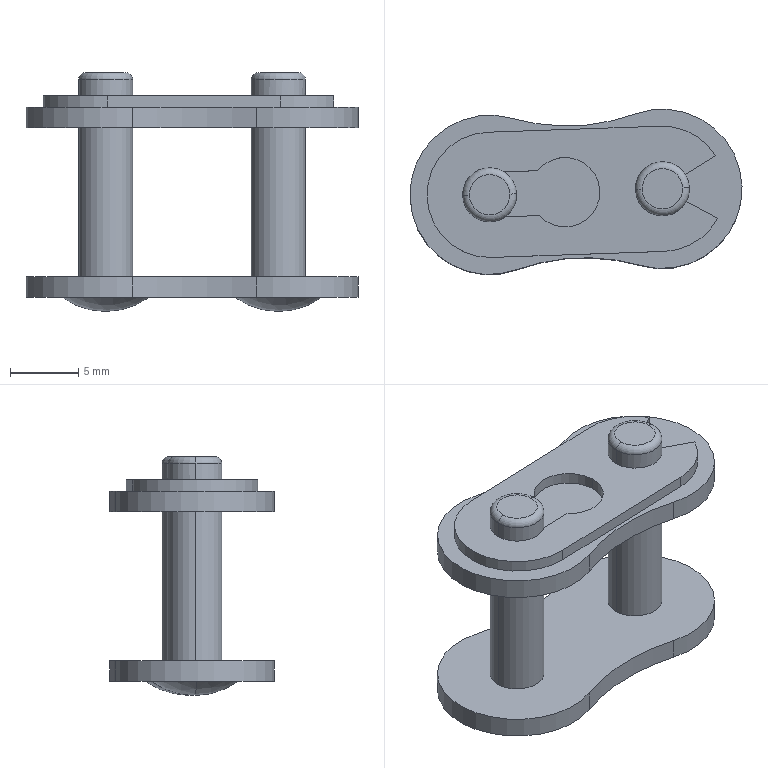Part | STEP file | CHES40-46-Part-12 | 1 solid | 45 faces | box 24.392 x 12.143 x 17.55 mm | volume 1198 mm3 | cylinder 23 | plane 14 | torus 4 | sphere 4 | commonest cylinder face diameters 3.97 x8 11.7 x6 29.64 x4 9.2 x3 5.1 x2
STEP:
#1=CARTESIAN_POINT('',(-191.992,69.511,9.53));
#2=VERTEX_POINT('',#1);
#3=CARTESIAN_POINT('',(-189.024,69.615,9.53));
#4=VERTEX_POINT('',#3);
#5=CARTESIAN_POINT('',(-190.508,69.563,9.53));
#6=DIRECTION('',(0.,0.,1.));
#7=DIRECTION('',(0.9994,0.0349,0.));
#8=AXIS2_PLACEMENT_3D('',#5,#6,#7);
#9=CIRCLE('',#8,1.485);
#10=EDGE_CURVE('',#2,#4,#9,.T.);
#11=ORIENTED_EDGE('',*,*,#10,.F.);
#12=CARTESIAN_POINT('',(-192.492,69.494,9.03));
#13=VERTEX_POINT('',#12);
#14=CARTESIAN_POINT('',(-191.992,69.511,9.03));
#15=DIRECTION('',(0.0349,-0.9994,0.));
#16=DIRECTION('',(0.9994,0.0349,0.));
#17=AXIS2_PLACEMENT_3D('',#14,#15,#16);
#18=CIRCLE('',#17,0.5);
#19=EDGE_CURVE('',#2,#13,#18,.T.);
#20=ORIENTED_EDGE('',*,*,#19,.T.);
#21=CARTESIAN_POINT('',(-188.524,69.632,9.03));
#22=VERTEX_POINT('',#21);
#23=CARTESIAN_POINT('',(-190.508,69.563,9.03));
#24=DIRECTION('',(0.,0.,-1.));
#25=DIRECTION('',(0.9994,0.0349,0.));
#26=AXIS2_PLACEMENT_3D('',#23,#24,#25);
#27=CIRCLE('',#26,1.985);
#28=EDGE_CURVE('',#22,#13,#27,.T.);
#29=ORIENTED_EDGE('',*,*,#28,.F.);
#30=CARTESIAN_POINT('',(-189.024,69.615,9.03));
#31=DIRECTION('',(-0.0349,0.9994,0.));
#32=DIRECTION('',(-0.9994,-0.0349,0.));
#33=AXIS2_PLACEMENT_3D('',#30,#31,#32);
#34=CIRCLE('',#33,0.5);
#35=EDGE_CURVE('',#4,#22,#34,.T.);
#36=ORIENTED_EDGE('',*,*,#35,.F.);
#37=EDGE_LOOP('',(#11,#20,#29,#36));
#38=FACE_OUTER_BOUND('',#37,.T.);
#39=CARTESIAN_POINT('',(-190.508,69.563,9.03));
#40=DIRECTION('',(0.,0.,-1.));
#41=DIRECTION('',(0.9994,0.0349,0.));
#42=AXIS2_PLACEMENT_3D('',#39,#40,#41);
#43=TOROIDAL_SURFACE('',#42,1.485,0.5);
#44=ADVANCED_FACE('',(#38),#43,.T.);
#45=CARTESIAN_POINT('',(-204.684,69.068,9.53));
#46=VERTEX_POINT('',#45);
#47=CARTESIAN_POINT('',(-201.716,69.172,9.53));
#48=VERTEX_POINT('',#47);
#49=CARTESIAN_POINT('',(-203.2,69.12,9.53));
#50=DIRECTION('',(0.,0.,1.));
#51=DIRECTION('',(0.9994,0.0349,0.));
#52=AXIS2_PLACEMENT_3D('',#49,#50,#51);
#53=CIRCLE('',#52,1.485);
#54=EDGE_CURVE('',#46,#48,#53,.T.);
#55=ORIENTED_EDGE('',*,*,#54,.F.);
#56=CARTESIAN_POINT('',(-205.184,69.051,9.03));
#57=VERTEX_POINT('',#56);
#58=CARTESIAN_POINT('',(-204.684,69.068,9.03));
#59=DIRECTION('',(0.0349,-0.9994,0.));
#60=DIRECTION('',(0.9994,0.0349,0.));
#61=AXIS2_PLACEMENT_3D('',#58,#59,#60);
#62=CIRCLE('',#61,0.5);
#63=EDGE_CURVE('',#46,#57,#62,.T.);
#64=ORIENTED_EDGE('',*,*,#63,.T.);
#65=CARTESIAN_POINT('',(-201.216,69.189,9.03));
#66=VERTEX_POINT('',#65);
#67=CARTESIAN_POINT('',(-203.2,69.12,9.03));
#68=DIRECTION('',(0.,0.,-1.));
#69=DIRECTION('',(0.9994,0.0349,0.));
#70=AXIS2_PLACEMENT_3D('',#67,#68,#69);
#71=CIRCLE('',#70,1.985);
#72=EDGE_CURVE('',#66,#57,#71,.T.);
#73=ORIENTED_EDGE('',*,*,#72,.F.);
#74=CARTESIAN_POINT('',(-201.716,69.172,9.03));
#75=DIRECTION('',(-0.0349,0.9994,0.));
#76=DIRECTION('',(-0.9994,-0.0349,0.));
#77=AXIS2_PLACEMENT_3D('',#74,#75,#76);
#78=CIRCLE('',#77,0.5);
#79=EDGE_CURVE('',#48,#66,#78,.T.);
#80=ORIENTED_EDGE('',*,*,#79,.F.);
#81=EDGE_LOOP('',(#55,#64,#73,#80));
#82=FACE_OUTER_BOUND('',#81,.T.);
#83=CARTESIAN_POINT('',(-203.2,69.12,9.03));
#84=DIRECTION('',(0.,0.,-1.));
#85=DIRECTION('',(0.9994,0.0349,0.));
#86=AXIS2_PLACEMENT_3D('',#83,#84,#85);
#87=TOROIDAL_SURFACE('',#86,1.485,0.5);
#88=ADVANCED_FACE('',(#82),#87,.T.);
#89=ORIENTED_EDGE('',*,*,#72,.T.);
#90=CARTESIAN_POINT('',(-205.184,69.051,7.825));
#91=VERTEX_POINT('',#90);
#92=CARTESIAN_POINT('',(-205.184,69.051,-8.02));
#93=DIRECTION('',(0.,0.,-1.));
#94=VECTOR('',#93,1000.);
#95=LINE('',#92,#94);
#96=EDGE_CURVE('',#57,#91,#95,.T.);
#97=ORIENTED_EDGE('',*,*,#96,.T.);
#98=CARTESIAN_POINT('',(-202.04,67.51,7.825));
#99=VERTEX_POINT('',#98);
#100=CARTESIAN_POINT('',(-203.2,69.12,7.825));
#101=DIRECTION('',(0.,0.,1.));
#102=DIRECTION('',(-0.9994,-0.0349,0.));
#103=AXIS2_PLACEMENT_3D('',#100,#101,#102);
#104=CIRCLE('',#103,1.985);
#105=EDGE_CURVE('',#91,#99,#104,.T.);
#106=ORIENTED_EDGE('',*,*,#105,.T.);
#107=CARTESIAN_POINT('',(-202.04,67.51,6.975));
#108=VERTEX_POINT('',#107);
#109=CARTESIAN_POINT('',(-202.04,67.51,7.825));
#110=DIRECTION('',(0.,0.,-1.));
#111=VECTOR('',#110,1000.);
#112=LINE('',#109,#111);
#113=EDGE_CURVE('',#99,#108,#112,.T.);
#114=ORIENTED_EDGE('',*,*,#113,.T.);
#115=CARTESIAN_POINT('',(-201.216,69.189,6.975));
#116=VERTEX_POINT('',#115);
#117=CARTESIAN_POINT('',(-203.2,69.12,6.975));
#118=DIRECTION('',(0.,0.,1.));
#119=DIRECTION('',(0.9994,0.0349,0.));
#120=AXIS2_PLACEMENT_3D('',#117,#118,#119);
#121=CIRCLE('',#120,1.985);
#122=EDGE_CURVE('',#108,#116,#121,.T.);
#123=ORIENTED_EDGE('',*,*,#122,.T.);
#124=CARTESIAN_POINT('',(-201.216,69.189,-8.02));
#125=DIRECTION('',(0.,0.,-1.));
#126=VECTOR('',#125,1000.);
#127=LINE('',#124,#126);
#128=EDGE_CURVE('',#66,#116,#127,.T.);
#129=ORIENTED_EDGE('',*,*,#128,.F.);
#130=EDGE_LOOP('',(#89,#97,#106,#114,#123,#129));
#131=FACE_OUTER_BOUND('',#130,.T.);
#132=CARTESIAN_POINT('',(-203.2,69.12,-8.02));
#133=DIRECTION('',(0.,0.,-1.));
#134=DIRECTION('',(0.9994,0.0349,0.));
#135=AXIS2_PLACEMENT_3D('',#132,#133,#134);
#136=CYLINDRICAL_SURFACE('',#135,1.985);
#137=ADVANCED_FACE('',(#131),#136,.T.);
#138=CARTESIAN_POINT('',(-199.539,67.597,7.825));
#139=VERTEX_POINT('',#138);
#140=CARTESIAN_POINT('',(-195.105,69.403,7.825));
#141=VERTEX_POINT('',#140);
#142=CARTESIAN_POINT('',(-197.653,69.314,7.825));
#143=DIRECTION('',(0.,0.,1.));
#144=DIRECTION('',(-0.9994,-0.0349,0.));
#145=AXIS2_PLACEMENT_3D('',#142,#143,#144);
#146=CIRCLE('',#145,2.55);
#147=EDGE_CURVE('',#139,#141,#146,.T.);
#148=ORIENTED_EDGE('',*,*,#147,.T.);
#149=CARTESIAN_POINT('',(-195.105,69.403,6.975));
#150=VERTEX_POINT('',#149);
#151=CARTESIAN_POINT('',(-195.105,69.403,7.825));
#152=DIRECTION('',(0.,0.,-1.));
#153=VECTOR('',#152,1000.);
#154=LINE('',#151,#153);
#155=EDGE_CURVE('',#141,#150,#154,.T.);
#156=ORIENTED_EDGE('',*,*,#155,.T.);
#157=CARTESIAN_POINT('',(-199.539,67.597,6.975));
#158=VERTEX_POINT('',#157);
#159=CARTESIAN_POINT('',(-197.653,69.314,6.975));
#160=DIRECTION('',(0.,0.,1.));
#161=DIRECTION('',(-0.9994,-0.0349,0.));
#162=AXIS2_PLACEMENT_3D('',#159,#160,#161);
#163=CIRCLE('',#162,2.55);
#164=EDGE_CURVE('',#158,#150,#163,.T.);
#165=ORIENTED_EDGE('',*,*,#164,.F.);
#166=CARTESIAN_POINT('',(-199.539,67.597,7.825));
#167=DIRECTION('',(0.,0.,-1.));
#168=VECTOR('',#167,1000.);
#169=LINE('',#166,#168);
#170=EDGE_CURVE('',#139,#158,#169,.T.);
#171=ORIENTED_EDGE('',*,*,#170,.F.);
#172=EDGE_LOOP('',(#148,#156,#165,#171));
#173=FACE_OUTER_BOUND('',#172,.T.);
#174=CARTESIAN_POINT('',(-197.653,69.314,7.825));
#175=DIRECTION('',(0.,0.,-1.));
#176=DIRECTION('',(0.9994,0.0349,0.));
#177=AXIS2_PLACEMENT_3D('',#174,#175,#176);
#178=CYLINDRICAL_SURFACE('',#177,2.55);
#179=ADVANCED_FACE('',(#173),#178,.F.);
#180=CARTESIAN_POINT('',(-187.31,69.675,-6.975));
#181=VERTEX_POINT('',#180);
#182=CARTESIAN_POINT('',(-193.706,69.452,-6.975));
#183=VERTEX_POINT('',#182);
#184=CARTESIAN_POINT('',(-190.508,69.563,-6.975));
#185=DIRECTION('',(0.,0.,1.));
#186=DIRECTION('',(-0.9994,-0.0349,0.));
#187=AXIS2_PLACEMENT_3D('',#184,#185,#186);
#188=CIRCLE('',#187,3.2);
#189=EDGE_CURVE('',#181,#183,#188,.T.);
#190=ORIENTED_EDGE('',*,*,#189,.F.);
#191=CARTESIAN_POINT('',(-190.508,69.563,-8.02));
#192=VERTEX_POINT('',#191);
#193=CARTESIAN_POINT('',(-190.508,69.563,-2.598));
#194=DIRECTION('',(-0.0349,0.9994,0.));
#195=DIRECTION('',(-0.9994,-0.0349,0.));
#196=AXIS2_PLACEMENT_3D('',#193,#194,#195);
#197=CIRCLE('',#196,5.422);
#198=EDGE_CURVE('',#181,#192,#197,.T.);
#199=ORIENTED_EDGE('',*,*,#198,.T.);
#200=CARTESIAN_POINT('',(-190.508,69.563,-2.598));
#201=DIRECTION('',(0.0349,-0.9994,0.));
#202=DIRECTION('',(0.9994,0.0349,0.));
#203=AXIS2_PLACEMENT_3D('',#200,#201,#202);
#204=CIRCLE('',#203,5.422);
#205=EDGE_CURVE('',#183,#192,#204,.T.);
#206=ORIENTED_EDGE('',*,*,#205,.F.);
#207=EDGE_LOOP('',(#190,#199,#206));
#208=FACE_OUTER_BOUND('',#207,.T.);
#209=CARTESIAN_POINT('',(-190.508,69.563,-2.598));
#210=DIRECTION('',(-0.0349,0.9994,0.));
#211=DIRECTION('',(-0.9994,-0.0349,0.));
#212=AXIS2_PLACEMENT_3D('',#209,#210,#211);
#213=SPHERICAL_SURFACE('',#212,5.422);
#214=ADVANCED_FACE('',(#208),#213,.T.);
#215=CARTESIAN_POINT('',(-200.002,69.232,-6.975));
#216=VERTEX_POINT('',#215);
#217=CARTESIAN_POINT('',(-206.398,69.008,-6.975));
#218=VERTEX_POINT('',#217);
#219=CARTESIAN_POINT('',(-203.2,69.12,-6.975));
#220=DIRECTION('',(0.,0.,1.));
#221=DIRECTION('',(-0.9994,-0.0349,0.));
#222=AXIS2_PLACEMENT_3D('',#219,#220,#221);
#223=CIRCLE('',#222,3.2);
#224=EDGE_CURVE('',#216,#218,#223,.T.);
#225=ORIENTED_EDGE('',*,*,#224,.F.);
#226=CARTESIAN_POINT('',(-203.2,69.12,-8.02));
#227=VERTEX_POINT('',#226);
#228=CARTESIAN_POINT('',(-203.2,69.12,-2.598));
#229=DIRECTION('',(-0.0349,0.9994,0.));
#230=DIRECTION('',(-0.9994,-0.0349,0.));
#231=AXIS2_PLACEMENT_3D('',#228,#229,#230);
#232=CIRCLE('',#231,5.422);
#233=EDGE_CURVE('',#216,#227,#232,.T.);
#234=ORIENTED_EDGE('',*,*,#233,.T.);
#235=CARTESIAN_POINT('',(-203.2,69.12,-2.598));
#236=DIRECTION('',(0.0349,-0.9994,0.));
#237=DIRECTION('',(0.9994,0.0349,0.));
#238=AXIS2_PLACEMENT_3D('',#235,#236,#237);
#239=CIRCLE('',#238,5.422);
#240=EDGE_CURVE('',#218,#227,#239,.T.);
#241=ORIENTED_EDGE('',*,*,#240,.F.);
#242=EDGE_LOOP('',(#225,#234,#241));
#243=FACE_OUTER_BOUND('',#242,.T.);
#244=CARTESIAN_POINT('',(-203.2,69.12,-2.598));
#245=DIRECTION('',(-0.0349,0.9994,0.));
#246=DIRECTION('',(-0.9994,-0.0349,0.));
#247=AXIS2_PLACEMENT_3D('',#244,#245,#246);
#248=SPHERICAL_SURFACE('',#247,5.422);
#249=ADVANCED_FACE('',(#243),#248,.T.);
#250=CARTESIAN_POINT('',(-184.661,69.767,-5.475));
#251=VERTEX_POINT('',#250);
#252=CARTESIAN_POINT('',(-192.498,75.064,-5.475));
#253=VERTEX_POINT('',#252);
#254=CARTESIAN_POINT('',(-190.508,69.563,-5.475));
#255=DIRECTION('',(0.,0.,1.));
#256=DIRECTION('',(-0.9994,-0.0349,0.));
#257=AXIS2_PLACEMENT_3D('',#254,#255,#256);
#258=CIRCLE('',#257,5.85);
#259=EDGE_CURVE('',#251,#253,#258,.T.);
#260=ORIENTED_EDGE('',*,*,#259,.F.);
#261=CARTESIAN_POINT('',(-184.661,69.767,-6.975));
#262=VERTEX_POINT('',#261);
#263=CARTESIAN_POINT('',(-184.661,69.767,-5.475));
#264=DIRECTION('',(0.,0.,-1.));
#265=VECTOR('',#264,1000.);
#266=LINE('',#263,#265);
#267=EDGE_CURVE('',#251,#262,#266,.T.);
#268=ORIENTED_EDGE('',*,*,#267,.T.);
#269=CARTESIAN_POINT('',(-192.498,75.064,-6.975));
#270=VERTEX_POINT('',#269);
#271=CARTESIAN_POINT('',(-190.508,69.563,-6.975));
#272=DIRECTION('',(0.,0.,1.));
#273=DIRECTION('',(-0.9994,-0.0349,0.));
#274=AXIS2_PLACEMENT_3D('',#271,#272,#273);
#275=CIRCLE('',#274,5.85);
#276=EDGE_CURVE('',#262,#270,#275,.T.);
#277=ORIENTED_EDGE('',*,*,#276,.T.);
#278=CARTESIAN_POINT('',(-192.498,75.064,-5.475));
#279=DIRECTION('',(0.,0.,-1.));
#280=VECTOR('',#279,1000.);
#281=LINE('',#278,#280);
#282=EDGE_CURVE('',#253,#270,#281,.T.);
#283=ORIENTED_EDGE('',*,*,#282,.F.);
#284=EDGE_LOOP('',(#260,#268,#277,#283));
#285=FACE_OUTER_BOUND('',#284,.T.);
#286=CARTESIAN_POINT('',(-190.508,69.563,-5.475));
#287=DIRECTION('',(0.,0.,-1.));
#288=DIRECTION('',(0.9994,0.0349,0.));
#289=AXIS2_PLACEMENT_3D('',#286,#287,#288);
#290=CYLINDRICAL_SURFACE('',#289,5.85);
#291=ADVANCED_FACE('',(#285),#290,.T.);
#292=CARTESIAN_POINT('',(-201.216,69.189,5.475));
#293=VERTEX_POINT('',#292);
#294=CARTESIAN_POINT('',(-205.184,69.051,5.475));
#295=VERTEX_POINT('',#294);
#296=CARTESIAN_POINT('',(-203.2,69.12,5.475));
#297=DIRECTION('',(0.,0.,-1.));
#298=DIRECTION('',(0.9994,0.0349,0.));
#299=AXIS2_PLACEMENT_3D('',#296,#297,#298);
#300=CIRCLE('',#299,1.985);
#301=EDGE_CURVE('',#293,#295,#300,.T.);
#302=ORIENTED_EDGE('',*,*,#301,.T.);
#303=CARTESIAN_POINT('',(-205.184,69.051,-5.475));
#304=VERTEX_POINT('',#303);
#305=CARTESIAN_POINT('',(-205.184,69.051,-8.02));
#306=DIRECTION('',(0.,0.,-1.));
#307=VECTOR('',#306,1000.);
#308=LINE('',#305,#307);
#309=EDGE_CURVE('',#295,#304,#308,.T.);
#310=ORIENTED_EDGE('',*,*,#309,.T.);
#311=CARTESIAN_POINT('',(-201.216,69.189,-5.475));
#312=VERTEX_POINT('',#311);
#313=CARTESIAN_POINT('',(-203.2,69.12,-5.475));
#314=DIRECTION('',(0.,0.,1.));
#315=DIRECTION('',(-0.9994,-0.0349,0.));
#316=AXIS2_PLACEMENT_3D('',#313,#314,#315);
#317=CIRCLE('',#316,1.985);
#318=EDGE_CURVE('',#304,#312,#317,.T.);
#319=ORIENTED_EDGE('',*,*,#318,.T.);
#320=CARTESIAN_POINT('',(-201.216,69.189,-8.02));
#321=DIRECTION('',(0.,0.,-1.));
#322=VECTOR('',#321,1000.);
#323=LINE('',#320,#322);
#324=EDGE_CURVE('',#293,#312,#323,.T.);
#325=ORIENTED_EDGE('',*,*,#324,.F.);
#326=EDGE_LOOP('',(#302,#310,#319,#325));
#327=FACE_OUTER_BOUND('',#326,.T.);
#328=CARTESIAN_POINT('',(-203.2,69.12,-8.02));
#329=DIRECTION('',(0.,0.,-1.));
#330=DIRECTION('',(0.9994,0.0349,0.));
#331=AXIS2_PLACEMENT_3D('',#328,#329,#330);
#332=CYLINDRICAL_SURFACE('',#331,1.985);
#333=ADVANCED_FACE('',(#327),#332,.T.);
#334=ORIENTED_EDGE('',*,*,#28,.T.);
#335=CARTESIAN_POINT('',(-192.492,69.494,7.825));
#336=VERTEX_POINT('',#335);
#337=CARTESIAN_POINT('',(-192.492,69.494,-8.02));
#338=DIRECTION('',(0.,0.,-1.));
#339=VECTOR('',#338,1000.);
#340=LINE('',#337,#339);
#341=EDGE_CURVE('',#13,#336,#340,.T.);
#342=ORIENTED_EDGE('',*,*,#341,.T.);
#343=CARTESIAN_POINT('',(-188.755,68.631,7.825));
#344=VERTEX_POINT('',#343);
#345=CARTESIAN_POINT('',(-190.508,69.563,7.825));
#346=DIRECTION('',(0.,0.,1.));
#347=DIRECTION('',(-0.9994,-0.0349,0.));
#348=AXIS2_PLACEMENT_3D('',#345,#346,#347);
#349=CIRCLE('',#348,1.985);
#350=EDGE_CURVE('',#336,#344,#349,.T.);
#351=ORIENTED_EDGE('',*,*,#350,.T.);
#352=CARTESIAN_POINT('',(-188.755,68.631,6.975));
#353=VERTEX_POINT('',#352);
#354=CARTESIAN_POINT('',(-188.755,68.631,7.825));
#355=DIRECTION('',(0.,0.,-1.));
#356=VECTOR('',#355,1000.);
#357=LINE('',#354,#356);
#358=EDGE_CURVE('',#344,#353,#357,.T.);
#359=ORIENTED_EDGE('',*,*,#358,.T.);
#360=CARTESIAN_POINT('',(-188.524,69.632,6.975));
#361=VERTEX_POINT('',#360);
#362=CARTESIAN_POINT('',(-190.508,69.563,6.975));
#363=DIRECTION('',(0.,0.,-1.));
#364=DIRECTION('',(0.9994,0.0349,0.));
#365=AXIS2_PLACEMENT_3D('',#362,#363,#364);
#366=CIRCLE('',#365,1.985);
#367=EDGE_CURVE('',#361,#353,#366,.T.);
#368=ORIENTED_EDGE('',*,*,#367,.F.);
#369=CARTESIAN_POINT('',(-188.524,69.632,-8.02));
#370=DIRECTION('',(0.,0.,-1.));
#371=VECTOR('',#370,1000.);
#372=LINE('',#369,#371);
#373=EDGE_CURVE('',#22,#361,#372,.T.);
#374=ORIENTED_EDGE('',*,*,#373,.F.);
#375=EDGE_LOOP('',(#334,#342,#351,#359,#368,#374));
#376=FACE_OUTER_BOUND('',#375,.T.);
#377=CARTESIAN_POINT('',(-190.508,69.563,-8.02));
#378=DIRECTION('',(0.,0.,-1.));
#379=DIRECTION('',(0.9994,0.0349,0.));
#380=AXIS2_PLACEMENT_3D('',#377,#378,#379);
#381=CYLINDRICAL_SURFACE('',#380,1.985);
#382=ADVANCED_FACE('',(#376),#381,.T.);
#383=CARTESIAN_POINT('',(-192.11,63.937,5.475));
#384=VERTEX_POINT('',#383);
#385=CARTESIAN_POINT('',(-184.661,69.767,5.475));
#386=VERTEX_POINT('',#385);
#387=CARTESIAN_POINT('',(-190.508,69.563,5.475));
#388=DIRECTION('',(0.,0.,1.));
#389=DIRECTION('',(-0.9994,-0.0349,0.));
#390=AXIS2_PLACEMENT_3D('',#387,#388,#389);
#391=CIRCLE('',#390,5.85);
#392=EDGE_CURVE('',#384,#386,#391,.T.);
#393=ORIENTED_EDGE('',*,*,#392,.T.);
#394=CARTESIAN_POINT('',(-184.661,69.767,6.975));
#395=VERTEX_POINT('',#394);
#396=CARTESIAN_POINT('',(-184.661,69.767,5.475));
#397=DIRECTION('',(0.,0.,1.));
#398=VECTOR('',#397,1000.);
#399=LINE('',#396,#398);
#400=EDGE_CURVE('',#386,#395,#399,.T.);
#401=ORIENTED_EDGE('',*,*,#400,.T.);
#402=CARTESIAN_POINT('',(-192.11,63.937,6.975));
#403=VERTEX_POINT('',#402);
#404=CARTESIAN_POINT('',(-190.508,69.563,6.975));
#405=DIRECTION('',(0.,0.,1.));
#406=DIRECTION('',(-0.9994,-0.0349,0.));
#407=AXIS2_PLACEMENT_3D('',#404,#405,#406);
#408=CIRCLE('',#407,5.85);
#409=EDGE_CURVE('',#403,#395,#408,.T.);
#410=ORIENTED_EDGE('',*,*,#409,.F.);
#411=CARTESIAN_POINT('',(-192.11,63.937,5.475));
#412=DIRECTION('',(0.,0.,1.));
#413=VECTOR('',#412,1000.);
#414=LINE('',#411,#413);
#415=EDGE_CURVE('',#384,#403,#414,.T.);
#416=ORIENTED_EDGE('',*,*,#415,.F.);
#417=EDGE_LOOP('',(#393,#401,#410,#416));
#418=FACE_OUTER_BOUND('',#417,.T.);
#419=CARTESIAN_POINT('',(-190.508,69.563,5.475));
#420=DIRECTION('',(0.,0.,1.));
#421=DIRECTION('',(0.9994,0.0349,0.));
#422=AXIS2_PLACEMENT_3D('',#419,#420,#421);
#423=CYLINDRICAL_SURFACE('',#422,5.85);
#424=ADVANCED_FACE('',(#418),#423,.T.);
#425=CARTESIAN_POINT('',(-188.524,69.632,5.475));
#426=VERTEX_POINT('',#425);
#427=CARTESIAN_POINT('',(-192.492,69.494,5.475));
#428=VERTEX_POINT('',#427);
#429=CARTESIAN_POINT('',(-190.508,69.563,5.475));
#430=DIRECTION('',(0.,0.,-1.));
#431=DIRECTION('',(0.9994,0.0349,0.));
#432=AXIS2_PLACEMENT_3D('',#429,#430,#431);
#433=CIRCLE('',#432,1.985);
#434=EDGE_CURVE('',#426,#428,#433,.T.);
#435=ORIENTED_EDGE('',*,*,#434,.T.);
#436=CARTESIAN_POINT('',(-192.492,69.494,-5.475));
#437=VERTEX_POINT('',#436);
#438=CARTESIAN_POINT('',(-192.492,69.494,-8.02));
#439=DIRECTION('',(0.,0.,-1.));
#440=VECTOR('',#439,1000.);
#441=LINE('',#438,#440);
#442=EDGE_CURVE('',#428,#437,#441,.T.);
#443=ORIENTED_EDGE('',*,*,#442,.T.);
#444=CARTESIAN_POINT('',(-188.524,69.632,-5.475));
#445=VERTEX_POINT('',#444);
#446=CARTESIAN_POINT('',(-190.508,69.563,-5.475));
#447=DIRECTION('',(0.,0.,1.));
#448=DIRECTION('',(-0.9994,-0.0349,0.));
#449=AXIS2_PLACEMENT_3D('',#446,#447,#448);
#450=CIRCLE('',#449,1.985);
#451=EDGE_CURVE('',#437,#445,#450,.T.);
#452=ORIENTED_EDGE('',*,*,#451,.T.);
#453=CARTESIAN_POINT('',(-188.524,69.632,-8.02));
#454=DIRECTION('',(0.,0.,-1.));
#455=VECTOR('',#454,1000.);
#456=LINE('',#453,#455);
#457=EDGE_CURVE('',#426,#445,#456,.T.);
#458=ORIENTED_EDGE('',*,*,#457,.F.);
#459=EDGE_LOOP('',(#435,#443,#452,#458));
#460=FACE_OUTER_BOUND('',#459,.T.);
#461=CARTESIAN_POINT('',(-190.508,69.563,-8.02));
#462=DIRECTION('',(0.,0.,-1.));
#463=DIRECTION('',(0.9994,0.0349,0.));
#464=AXIS2_PLACEMENT_3D('',#461,#462,#463);
#465=CYLINDRICAL_SURFACE('',#464,1.985);
#466=ADVANCED_FACE('',(#460),#465,.T.);
#467=ORIENTED_EDGE('',*,*,#409,.T.);
#468=CARTESIAN_POINT('',(-192.498,75.064,6.975));
#469=VERTEX_POINT('',#468);
#470=CARTESIAN_POINT('',(-190.508,69.563,6.975));
#471=DIRECTION('',(0.,0.,1.));
#472=DIRECTION('',(-0.9994,-0.0349,0.));
#473=AXIS2_PLACEMENT_3D('',#470,#471,#472);
#474=CIRCLE('',#473,5.85);
#475=EDGE_CURVE('',#395,#469,#474,.T.);
#476=ORIENTED_EDGE('',*,*,#475,.T.);
#477=CARTESIAN_POINT('',(-201.598,74.746,6.975));
#478=VERTEX_POINT('',#477);
#479=CARTESIAN_POINT('',(-197.54,89.,6.975));
#480=DIRECTION('',(0.,0.,-1.));
#481=DIRECTION('',(0.9994,0.0349,0.));
#482=AXIS2_PLACEMENT_3D('',#479,#480,#481);
#483=CIRCLE('',#482,14.82);
#484=EDGE_CURVE('',#469,#478,#483,.T.);
#485=ORIENTED_EDGE('',*,*,#484,.T.);
#486=CARTESIAN_POINT('',(-201.21,63.619,6.975));
#487=VERTEX_POINT('',#486);
#488=CARTESIAN_POINT('',(-203.2,69.12,6.975));
#489=DIRECTION('',(0.,0.,1.));
#490=DIRECTION('',(0.9994,0.0349,0.));
#491=AXIS2_PLACEMENT_3D('',#488,#489,#490);
#492=CIRCLE('',#491,5.85);
#493=EDGE_CURVE('',#478,#487,#492,.T.);
#494=ORIENTED_EDGE('',*,*,#493,.T.);
#495=CARTESIAN_POINT('',(-196.167,49.683,6.975));
#496=DIRECTION('',(0.,0.,-1.));
#497=DIRECTION('',(-0.9994,-0.0349,0.));
#498=AXIS2_PLACEMENT_3D('',#495,#496,#497);
#499=CIRCLE('',#498,14.82);
#500=EDGE_CURVE('',#487,#403,#499,.T.);
#501=ORIENTED_EDGE('',*,*,#500,.T.);
#502=EDGE_LOOP('',(#467,#476,#485,#494,#501));
#503=FACE_OUTER_BOUND('',#502,.T.);
#504=CARTESIAN_POINT('',(-186.446,67.404,6.975));
#505=VERTEX_POINT('',#504);
#506=CARTESIAN_POINT('',(-186.446,67.404,6.975));
#507=DIRECTION('',(-0.8829,0.4695,0.));
#508=VECTOR('',#507,1000.);
#509=LINE('',#506,#508);
#510=EDGE_CURVE('',#505,#353,#509,.T.);
#511=ORIENTED_EDGE('',*,*,#510,.F.);
#512=CARTESIAN_POINT('',(-190.347,64.966,6.975));
#513=VERTEX_POINT('',#512);
#514=CARTESIAN_POINT('',(-190.508,69.563,6.975));
#515=DIRECTION('',(0.,0.,1.));
#516=DIRECTION('',(-0.9994,-0.0349,0.));
#517=AXIS2_PLACEMENT_3D('',#514,#515,#516);
#518=CIRCLE('',#517,4.6);
#519=EDGE_CURVE('',#513,#505,#518,.T.);
#520=ORIENTED_EDGE('',*,*,#519,.F.);
#521=CARTESIAN_POINT('',(-203.039,64.523,6.975));
#522=VERTEX_POINT('',#521);
#523=CARTESIAN_POINT('',(-190.347,64.966,6.975));
#524=DIRECTION('',(0.9994,0.0349,0.));
#525=VECTOR('',#524,1000.);
#526=LINE('',#523,#525);
#527=EDGE_CURVE('',#522,#513,#526,.T.);
#528=ORIENTED_EDGE('',*,*,#527,.F.);
#529=CARTESIAN_POINT('',(-203.361,73.717,6.975));
#530=VERTEX_POINT('',#529);
#531=CARTESIAN_POINT('',(-203.2,69.12,6.975));
#532=DIRECTION('',(0.,0.,1.));
#533=DIRECTION('',(-0.9994,-0.0349,0.));
#534=AXIS2_PLACEMENT_3D('',#531,#532,#533);
#535=CIRCLE('',#534,4.6);
#536=EDGE_CURVE('',#530,#522,#535,.T.);
#537=ORIENTED_EDGE('',*,*,#536,.F.);
#538=CARTESIAN_POINT('',(-190.668,74.16,6.975));
#539=VERTEX_POINT('',#538);
#540=CARTESIAN_POINT('',(-190.668,74.16,6.975));
#541=DIRECTION('',(-0.9994,-0.0349,0.));
#542=VECTOR('',#541,1000.);
#543=LINE('',#540,#542);
#544=EDGE_CURVE('',#539,#530,#543,.T.);
#545=ORIENTED_EDGE('',*,*,#544,.F.);
#546=CARTESIAN_POINT('',(-186.607,72.001,6.975));
#547=VERTEX_POINT('',#546);
#548=CARTESIAN_POINT('',(-190.508,69.563,6.975));
#549=DIRECTION('',(0.,0.,1.));
#550=DIRECTION('',(-0.9994,-0.0349,0.));
#551=AXIS2_PLACEMENT_3D('',#548,#549,#550);
#552=CIRCLE('',#551,4.6);
#553=EDGE_CURVE('',#547,#539,#552,.T.);
#554=ORIENTED_EDGE('',*,*,#553,.F.);
#555=CARTESIAN_POINT('',(-188.824,70.615,6.975));
#556=VERTEX_POINT('',#555);
#557=CARTESIAN_POINT('',(-186.607,72.001,6.975));
#558=DIRECTION('',(0.848,0.5299,0.));
#559=VECTOR('',#558,1000.);
#560=LINE('',#557,#559);
#561=EDGE_CURVE('',#556,#547,#560,.T.);
#562=ORIENTED_EDGE('',*,*,#561,.F.);
#563=CARTESIAN_POINT('',(-190.508,69.563,6.975));
#564=DIRECTION('',(0.,0.,-1.));
#565=DIRECTION('',(0.9994,0.0349,0.));
#566=AXIS2_PLACEMENT_3D('',#563,#564,#565);
#567=CIRCLE('',#566,1.985);
#568=EDGE_CURVE('',#556,#361,#567,.T.);
#569=ORIENTED_EDGE('',*,*,#568,.T.);
#570=ORIENTED_EDGE('',*,*,#367,.T.);
#571=EDGE_LOOP('',(#511,#520,#528,#537,#545,#554,#562,#569,#570));
#572=FACE_BOUND('',#571,.T.);
#573=CARTESIAN_POINT('',(-194.024,79.282,6.975));
#574=DIRECTION('',(0.,0.,-1.));
#575=DIRECTION('',(-0.9994,-0.0349,0.));
#576=AXIS2_PLACEMENT_3D('',#573,#574,#575);
#577=PLANE('',#576);
#578=ADVANCED_FACE('',(#503,#572),#577,.F.);
#579=ORIENTED_EDGE('',*,*,#434,.F.);
#580=CARTESIAN_POINT('',(-190.508,69.563,5.475));
#581=DIRECTION('',(0.,0.,-1.));
#582=DIRECTION('',(0.9994,0.0349,0.));
#583=AXIS2_PLACEMENT_3D('',#580,#581,#582);
#584=CIRCLE('',#583,1.985);
#585=EDGE_CURVE('',#428,#426,#584,.T.);
#586=ORIENTED_EDGE('',*,*,#585,.F.);
#587=EDGE_LOOP('',(#579,#586));
#588=FACE_BOUND('',#587,.T.);
#589=ORIENTED_EDGE('',*,*,#392,.F.);
#590=CARTESIAN_POINT('',(-201.21,63.619,5.475));
#591=VERTEX_POINT('',#590);
#592=CARTESIAN_POINT('',(-196.167,49.683,5.475));
#593=DIRECTION('',(0.,0.,-1.));
#594=DIRECTION('',(-0.9994,-0.0349,0.));
#595=AXIS2_PLACEMENT_3D('',#592,#593,#594);
#596=CIRCLE('',#595,14.82);
#597=EDGE_CURVE('',#591,#384,#596,.T.);
#598=ORIENTED_EDGE('',*,*,#597,.F.);
#599=CARTESIAN_POINT('',(-201.598,74.746,5.475));
#600=VERTEX_POINT('',#599);
#601=CARTESIAN_POINT('',(-203.2,69.12,5.475));
#602=DIRECTION('',(0.,0.,1.));
#603=DIRECTION('',(0.9994,0.0349,0.));
#604=AXIS2_PLACEMENT_3D('',#601,#602,#603);
#605=CIRCLE('',#604,5.85);
#606=EDGE_CURVE('',#600,#591,#605,.T.);
#607=ORIENTED_EDGE('',*,*,#606,.F.);
#608=CARTESIAN_POINT('',(-192.498,75.064,5.475));
#609=VERTEX_POINT('',#608);
#610=CARTESIAN_POINT('',(-197.54,89.,5.475));
#611=DIRECTION('',(0.,0.,-1.));
#612=DIRECTION('',(0.9994,0.0349,0.));
#613=AXIS2_PLACEMENT_3D('',#610,#611,#612);
#614=CIRCLE('',#613,14.82);
#615=EDGE_CURVE('',#609,#600,#614,.T.);
#616=ORIENTED_EDGE('',*,*,#615,.F.);
#617=CARTESIAN_POINT('',(-190.508,69.563,5.475));
#618=DIRECTION('',(0.,0.,1.));
#619=DIRECTION('',(-0.9994,-0.0349,0.));
#620=AXIS2_PLACEMENT_3D('',#617,#618,#619);
#621=CIRCLE('',#620,5.85);
#622=EDGE_CURVE('',#386,#609,#621,.T.);
#623=ORIENTED_EDGE('',*,*,#622,.F.);
#624=EDGE_LOOP('',(#589,#598,#607,#616,#623));
#625=FACE_OUTER_BOUND('',#624,.T.);
#626=ORIENTED_EDGE('',*,*,#301,.F.);
#627=CARTESIAN_POINT('',(-203.2,69.12,5.475));
#628=DIRECTION('',(0.,0.,-1.));
#629=DIRECTION('',(0.9994,0.0349,0.));
#630=AXIS2_PLACEMENT_3D('',#627,#628,#629);
#631=CIRCLE('',#630,1.985);
#632=EDGE_CURVE('',#295,#293,#631,.T.);
#633=ORIENTED_EDGE('',*,*,#632,.F.);
#634=EDGE_LOOP('',(#626,#633));
#635=FACE_BOUND('',#634,.T.);
#636=CARTESIAN_POINT('',(-194.024,79.282,5.475));
#637=DIRECTION('',(0.,0.,-1.));
#638=DIRECTION('',(-0.9994,-0.0349,0.));
#639=AXIS2_PLACEMENT_3D('',#636,#637,#638);
#640=PLANE('',#639);
#641=ADVANCED_FACE('',(#588,#625,#635),#640,.T.);
#642=ORIENTED_EDGE('',*,*,#442,.F.);
#643=ORIENTED_EDGE('',*,*,#585,.T.);
#644=ORIENTED_EDGE('',*,*,#457,.T.);
#645=CARTESIAN_POINT('',(-190.508,69.563,-5.475));
#646=DIRECTION('',(0.,0.,1.));
#647=DIRECTION('',(-0.9994,-0.0349,0.));
#648=AXIS2_PLACEMENT_3D('',#645,#646,#647);
#649=CIRCLE('',#648,1.985);
#650=EDGE_CURVE('',#445,#437,#649,.T.);
#651=ORIENTED_EDGE('',*,*,#650,.T.);
#652=EDGE_LOOP('',(#642,#643,#644,#651));
#653=FACE_OUTER_BOUND('',#652,.T.);
#654=CARTESIAN_POINT('',(-190.508,69.563,-8.02));
#655=DIRECTION('',(0.,0.,-1.));
#656=DIRECTION('',(0.9994,0.0349,0.));
#657=AXIS2_PLACEMENT_3D('',#654,#655,#656);
#658=CYLINDRICAL_SURFACE('',#657,1.985);
#659=ADVANCED_FACE('',(#653),#658,.T.);
#660=ORIENTED_EDGE('',*,*,#400,.F.);
#661=ORIENTED_EDGE('',*,*,#622,.T.);
#662=CARTESIAN_POINT('',(-192.498,75.064,5.475));
#663=DIRECTION('',(0.,0.,1.));
#664=VECTOR('',#663,1000.);
#665=LINE('',#662,#664);
#666=EDGE_CURVE('',#609,#469,#665,.T.);
#667=ORIENTED_EDGE('',*,*,#666,.T.);
#668=ORIENTED_EDGE('',*,*,#475,.F.);
#669=EDGE_LOOP('',(#660,#661,#667,#668));
#670=FACE_OUTER_BOUND('',#669,.T.);
#671=CARTESIAN_POINT('',(-190.508,69.563,5.475));
#672=DIRECTION('',(0.,0.,1.));
#673=DIRECTION('',(0.9994,0.0349,0.));
#674=AXIS2_PLACEMENT_3D('',#671,#672,#673);
#675=CYLINDRICAL_SURFACE('',#674,5.85);
#676=ADVANCED_FACE('',(#670),#675,.T.);
#677=ORIENTED_EDGE('',*,*,#484,.F.);
#678=ORIENTED_EDGE('',*,*,#666,.F.);
#679=ORIENTED_EDGE('',*,*,#615,.T.);
#680=CARTESIAN_POINT('',(-201.598,74.746,5.475));
#681=DIRECTION('',(0.,0.,1.));
#682=VECTOR('',#681,1000.);
#683=LINE('',#680,#682);
#684=EDGE_CURVE('',#600,#478,#683,.T.);
#685=ORIENTED_EDGE('',*,*,#684,.T.);
#686=EDGE_LOOP('',(#677,#678,#679,#685));
#687=FACE_OUTER_BOUND('',#686,.T.);
#688=CARTESIAN_POINT('',(-197.54,89.,5.475));
#689=DIRECTION('',(0.,0.,1.));
#690=DIRECTION('',(0.9994,0.0349,0.));
#691=AXIS2_PLACEMENT_3D('',#688,#689,#690);
#692=CYLINDRICAL_SURFACE('',#691,14.82);
#693=ADVANCED_FACE('',(#687),#692,.F.);
#694=ORIENTED_EDGE('',*,*,#493,.F.);
#695=ORIENTED_EDGE('',*,*,#684,.F.);
#696=ORIENTED_EDGE('',*,*,#606,.T.);
#697=CARTESIAN_POINT('',(-201.21,63.619,5.475));
#698=DIRECTION('',(0.,0.,1.));
#699=VECTOR('',#698,1000.);
#700=LINE('',#697,#699);
#701=EDGE_CURVE('',#591,#487,#700,.T.);
#702=ORIENTED_EDGE('',*,*,#701,.T.);
#703=EDGE_LOOP('',(#694,#695,#696,#702));
#704=FACE_OUTER_BOUND('',#703,.T.);
#705=CARTESIAN_POINT('',(-203.2,69.12,5.475));
#706=DIRECTION('',(0.,0.,1.));
#707=DIRECTION('',(0.9994,0.0349,0.));
#708=AXIS2_PLACEMENT_3D('',#705,#706,#707);
#709=CYLINDRICAL_SURFACE('',#708,5.85);
#710=ADVANCED_FACE('',(#704),#709,.T.);
#711=ORIENTED_EDGE('',*,*,#500,.F.);
#712=ORIENTED_EDGE('',*,*,#701,.F.);
#713=ORIENTED_EDGE('',*,*,#597,.T.);
#714=ORIENTED_EDGE('',*,*,#415,.T.);
#715=EDGE_LOOP('',(#711,#712,#713,#714));
#716=FACE_OUTER_BOUND('',#715,.T.);
#717=CARTESIAN_POINT('',(-196.167,49.683,5.475));
#718=DIRECTION('',(0.,0.,1.));
#719=DIRECTION('',(0.9994,0.0349,0.));
#720=AXIS2_PLACEMENT_3D('',#717,#718,#719);
#721=CYLINDRICAL_SURFACE('',#720,14.82);
#722=ADVANCED_FACE('',(#716),#721,.F.);
#723=CARTESIAN_POINT('',(-190.508,69.563,9.53));
#724=DIRECTION('',(0.,0.,1.));
#725=DIRECTION('',(0.9994,0.0349,0.));
#726=AXIS2_PLACEMENT_3D('',#723,#724,#725);
#727=CIRCLE('',#726,1.485);
#728=EDGE_CURVE('',#4,#2,#727,.T.);
#729=ORIENTED_EDGE('',*,*,#728,.T.);
#730=ORIENTED_EDGE('',*,*,#10,.T.);
#731=EDGE_LOOP('',(#729,#730));
#732=FACE_OUTER_BOUND('',#731,.T.);
#733=CARTESIAN_POINT('',(-192.492,69.494,9.53));
#734=DIRECTION('',(0.,0.,-1.));
#735=DIRECTION('',(0.9994,0.0349,0.));
#736=AXIS2_PLACEMENT_3D('',#733,#734,#735);
#737=PLANE('',#736);
#738=ADVANCED_FACE('',(#732),#737,.F.);
#739=ORIENTED_EDGE('',*,*,#341,.F.);
#740=CARTESIAN_POINT('',(-190.508,69.563,9.03));
#741=DIRECTION('',(0.,0.,-1.));
#742=DIRECTION('',(0.9994,0.0349,0.));
#743=AXIS2_PLACEMENT_3D('',#740,#741,#742);
#744=CIRCLE('',#743,1.985);
#745=EDGE_CURVE('',#13,#22,#744,.T.);
#746=ORIENTED_EDGE('',*,*,#745,.T.);
#747=ORIENTED_EDGE('',*,*,#373,.T.);
#748=ORIENTED_EDGE('',*,*,#568,.F.);
#749=CARTESIAN_POINT('',(-188.824,70.615,7.825));
#750=VERTEX_POINT('',#749);
#751=CARTESIAN_POINT('',(-188.824,70.615,7.825));
#752=DIRECTION('',(0.,0.,-1.));
#753=VECTOR('',#752,1000.);
#754=LINE('',#751,#753);
#755=EDGE_CURVE('',#750,#556,#754,.T.);
#756=ORIENTED_EDGE('',*,*,#755,.F.);
#757=CARTESIAN_POINT('',(-190.508,69.563,7.825));
#758=DIRECTION('',(0.,0.,1.));
#759=DIRECTION('',(-0.9994,-0.0349,0.));
#760=AXIS2_PLACEMENT_3D('',#757,#758,#759);
#761=CIRCLE('',#760,1.985);
#762=EDGE_CURVE('',#750,#336,#761,.T.);
#763=ORIENTED_EDGE('',*,*,#762,.T.);
#764=EDGE_LOOP('',(#739,#746,#747,#748,#756,#763));
#765=FACE_OUTER_BOUND('',#764,.T.);
#766=CARTESIAN_POINT('',(-190.508,69.563,-8.02));
#767=DIRECTION('',(0.,0.,-1.));
#768=DIRECTION('',(0.9994,0.0349,0.));
#769=AXIS2_PLACEMENT_3D('',#766,#767,#768);
#770=CYLINDRICAL_SURFACE('',#769,1.985);
#771=ADVANCED_FACE('',(#765),#770,.T.);
#772=ORIENTED_EDGE('',*,*,#309,.F.);
#773=ORIENTED_EDGE('',*,*,#632,.T.);
#774=ORIENTED_EDGE('',*,*,#324,.T.);
#775=CARTESIAN_POINT('',(-203.2,69.12,-5.475));
#776=DIRECTION('',(0.,0.,1.));
#777=DIRECTION('',(-0.9994,-0.0349,0.));
#778=AXIS2_PLACEMENT_3D('',#775,#776,#777);
#779=CIRCLE('',#778,1.985);
#780=EDGE_CURVE('',#312,#304,#779,.T.);
#781=ORIENTED_EDGE('',*,*,#780,.T.);
#782=EDGE_LOOP('',(#772,#773,#774,#781));
#783=FACE_OUTER_BOUND('',#782,.T.);
#784=CARTESIAN_POINT('',(-203.2,69.12,-8.02));
#785=DIRECTION('',(0.,0.,-1.));
#786=DIRECTION('',(0.9994,0.0349,0.));
#787=AXIS2_PLACEMENT_3D('',#784,#785,#786);
#788=CYLINDRICAL_SURFACE('',#787,1.985);
#789=ADVANCED_FACE('',(#783),#788,.T.);
#790=CARTESIAN_POINT('',(-192.11,63.937,-5.475));
#791=VERTEX_POINT('',#790);
#792=CARTESIAN_POINT('',(-190.508,69.563,-5.475));
#793=DIRECTION('',(0.,0.,1.));
#794=DIRECTION('',(-0.9994,-0.0349,0.));
#795=AXIS2_PLACEMENT_3D('',#792,#793,#794);
#796=CIRCLE('',#795,5.85);
#797=EDGE_CURVE('',#791,#251,#796,.T.);
#798=ORIENTED_EDGE('',*,*,#797,.T.);
#799=ORIENTED_EDGE('',*,*,#259,.T.);
#800=CARTESIAN_POINT('',(-201.598,74.746,-5.475));
#801=VERTEX_POINT('',#800);
#802=CARTESIAN_POINT('',(-197.54,89.,-5.475));
#803=DIRECTION('',(0.,0.,-1.));
#804=DIRECTION('',(0.9994,0.0349,0.));
#805=AXIS2_PLACEMENT_3D('',#802,#803,#804);
#806=CIRCLE('',#805,14.82);
#807=EDGE_CURVE('',#253,#801,#806,.T.);
#808=ORIENTED_EDGE('',*,*,#807,.T.);
#809=CARTESIAN_POINT('',(-201.21,63.619,-5.475));
#810=VERTEX_POINT('',#809);
#811=CARTESIAN_POINT('',(-203.2,69.12,-5.475));
#812=DIRECTION('',(0.,0.,1.));
#813=DIRECTION('',(0.9994,0.0349,0.));
#814=AXIS2_PLACEMENT_3D('',#811,#812,#813);
#815=CIRCLE('',#814,5.85);
#816=EDGE_CURVE('',#801,#810,#815,.T.);
#817=ORIENTED_EDGE('',*,*,#816,.T.);
#818=CARTESIAN_POINT('',(-196.167,49.683,-5.475));
#819=DIRECTION('',(0.,0.,-1.));
#820=DIRECTION('',(-0.9994,-0.0349,0.));
#821=AXIS2_PLACEMENT_3D('',#818,#819,#820);
#822=CIRCLE('',#821,14.82);
#823=EDGE_CURVE('',#810,#791,#822,.T.);
#824=ORIENTED_EDGE('',*,*,#823,.T.);
#825=EDGE_LOOP('',(#798,#799,#808,#817,#824));
#826=FACE_OUTER_BOUND('',#825,.T.);
#827=ORIENTED_EDGE('',*,*,#780,.F.);
#828=ORIENTED_EDGE('',*,*,#318,.F.);
#829=EDGE_LOOP('',(#827,#828));
#830=FACE_BOUND('',#829,.T.);
#831=ORIENTED_EDGE('',*,*,#650,.F.);
#832=ORIENTED_EDGE('',*,*,#451,.F.);
#833=EDGE_LOOP('',(#831,#832));
#834=FACE_BOUND('',#833,.T.);
#835=CARTESIAN_POINT('',(-194.024,79.282,-5.475));
#836=DIRECTION('',(0.,0.,1.));
#837=DIRECTION('',(-0.9994,-0.0349,0.));
#838=AXIS2_PLACEMENT_3D('',#835,#836,#837);
#839=PLANE('',#838);
#840=ADVANCED_FACE('',(#826,#830,#834),#839,.T.);
#841=CARTESIAN_POINT('',(-192.11,63.937,-6.975));
#842=VERTEX_POINT('',#841);
#843=CARTESIAN_POINT('',(-190.508,69.563,-6.975));
#844=DIRECTION('',(0.,0.,1.));
#845=DIRECTION('',(-0.9994,-0.0349,0.));
#846=AXIS2_PLACEMENT_3D('',#843,#844,#845);
#847=CIRCLE('',#846,5.85);
#848=EDGE_CURVE('',#842,#262,#847,.T.);
#849=ORIENTED_EDGE('',*,*,#848,.F.);
#850=CARTESIAN_POINT('',(-201.21,63.619,-6.975));
#851=VERTEX_POINT('',#850);
#852=CARTESIAN_POINT('',(-196.167,49.683,-6.975));
#853=DIRECTION('',(0.,0.,-1.));
#854=DIRECTION('',(-0.9994,-0.0349,0.));
#855=AXIS2_PLACEMENT_3D('',#852,#853,#854);
#856=CIRCLE('',#855,14.82);
#857=EDGE_CURVE('',#851,#842,#856,.T.);
#858=ORIENTED_EDGE('',*,*,#857,.F.);
#859=CARTESIAN_POINT('',(-201.598,74.746,-6.975));
#860=VERTEX_POINT('',#859);
#861=CARTESIAN_POINT('',(-203.2,69.12,-6.975));
#862=DIRECTION('',(0.,0.,1.));
#863=DIRECTION('',(0.9994,0.0349,0.));
#864=AXIS2_PLACEMENT_3D('',#861,#862,#863);
#865=CIRCLE('',#864,5.85);
#866=EDGE_CURVE('',#860,#851,#865,.T.);
#867=ORIENTED_EDGE('',*,*,#866,.F.);
#868=CARTESIAN_POINT('',(-197.54,89.,-6.975));
#869=DIRECTION('',(0.,0.,-1.));
#870=DIRECTION('',(0.9994,0.0349,0.));
#871=AXIS2_PLACEMENT_3D('',#868,#869,#870);
#872=CIRCLE('',#871,14.82);
#873=EDGE_CURVE('',#270,#860,#872,.T.);
#874=ORIENTED_EDGE('',*,*,#873,.F.);
#875=ORIENTED_EDGE('',*,*,#276,.F.);
#876=EDGE_LOOP('',(#849,#858,#867,#874,#875));
#877=FACE_OUTER_BOUND('',#876,.T.);
#878=CARTESIAN_POINT('',(-203.2,69.12,-6.975));
#879=DIRECTION('',(0.,0.,1.));
#880=DIRECTION('',(-0.9994,-0.0349,0.));
#881=AXIS2_PLACEMENT_3D('',#878,#879,#880);
#882=CIRCLE('',#881,3.2);
#883=EDGE_CURVE('',#218,#216,#882,.T.);
#884=ORIENTED_EDGE('',*,*,#883,.T.);
#885=ORIENTED_EDGE('',*,*,#224,.T.);
#886=EDGE_LOOP('',(#884,#885));
#887=FACE_BOUND('',#886,.T.);
#888=CARTESIAN_POINT('',(-190.508,69.563,-6.975));
#889=DIRECTION('',(0.,0.,1.));
#890=DIRECTION('',(-0.9994,-0.0349,0.));
#891=AXIS2_PLACEMENT_3D('',#888,#889,#890);
#892=CIRCLE('',#891,3.2);
#893=EDGE_CURVE('',#183,#181,#892,.T.);
#894=ORIENTED_EDGE('',*,*,#893,.T.);
#895=ORIENTED_EDGE('',*,*,#189,.T.);
#896=EDGE_LOOP('',(#894,#895));
#897=FACE_BOUND('',#896,.T.);
#898=CARTESIAN_POINT('',(-194.024,79.282,-6.975));
#899=DIRECTION('',(0.,0.,1.));
#900=DIRECTION('',(-0.9994,-0.0349,0.));
#901=AXIS2_PLACEMENT_3D('',#898,#899,#900);
#902=PLANE('',#901);
#903=ADVANCED_FACE('',(#877,#887,#897),#902,.F.);
#904=ORIENTED_EDGE('',*,*,#267,.F.);
#905=ORIENTED_EDGE('',*,*,#797,.F.);
#906=CARTESIAN_POINT('',(-192.11,63.937,-5.475));
#907=DIRECTION('',(0.,0.,-1.));
#908=VECTOR('',#907,1000.);
#909=LINE('',#906,#908);
#910=EDGE_CURVE('',#791,#842,#909,.T.);
#911=ORIENTED_EDGE('',*,*,#910,.T.);
#912=ORIENTED_EDGE('',*,*,#848,.T.);
#913=EDGE_LOOP('',(#904,#905,#911,#912));
#914=FACE_OUTER_BOUND('',#913,.T.);
#915=CARTESIAN_POINT('',(-190.508,69.563,-5.475));
#916=DIRECTION('',(0.,0.,-1.));
#917=DIRECTION('',(0.9994,0.0349,0.));
#918=AXIS2_PLACEMENT_3D('',#915,#916,#917);
#919=CYLINDRICAL_SURFACE('',#918,5.85);
#920=ADVANCED_FACE('',(#914),#919,.T.);
#921=ORIENTED_EDGE('',*,*,#873,.T.);
#922=CARTESIAN_POINT('',(-201.598,74.746,-5.475));
#923=DIRECTION('',(0.,0.,-1.));
#924=VECTOR('',#923,1000.);
#925=LINE('',#922,#924);
#926=EDGE_CURVE('',#801,#860,#925,.T.);
#927=ORIENTED_EDGE('',*,*,#926,.F.);
#928=ORIENTED_EDGE('',*,*,#807,.F.);
#929=ORIENTED_EDGE('',*,*,#282,.T.);
#930=EDGE_LOOP('',(#921,#927,#928,#929));
#931=FACE_OUTER_BOUND('',#930,.T.);
#932=CARTESIAN_POINT('',(-197.54,89.,-5.475));
#933=DIRECTION('',(0.,0.,-1.));
#934=DIRECTION('',(0.9994,0.0349,0.));
#935=AXIS2_PLACEMENT_3D('',#932,#933,#934);
#936=CYLINDRICAL_SURFACE('',#935,14.82);
#937=ADVANCED_FACE('',(#931),#936,.F.);
#938=ORIENTED_EDGE('',*,*,#866,.T.);
#939=CARTESIAN_POINT('',(-201.21,63.619,-5.475));
#940=DIRECTION('',(0.,0.,-1.));
#941=VECTOR('',#940,1000.);
#942=LINE('',#939,#941);
#943=EDGE_CURVE('',#810,#851,#942,.T.);
#944=ORIENTED_EDGE('',*,*,#943,.F.);
#945=ORIENTED_EDGE('',*,*,#816,.F.);
#946=ORIENTED_EDGE('',*,*,#926,.T.);
#947=EDGE_LOOP('',(#938,#944,#945,#946));
#948=FACE_OUTER_BOUND('',#947,.T.);
#949=CARTESIAN_POINT('',(-203.2,69.12,-5.475));
#950=DIRECTION('',(0.,0.,-1.));
#951=DIRECTION('',(0.9994,0.0349,0.));
#952=AXIS2_PLACEMENT_3D('',#949,#950,#951);
#953=CYLINDRICAL_SURFACE('',#952,5.85);
#954=ADVANCED_FACE('',(#948),#953,.T.);
#955=ORIENTED_EDGE('',*,*,#857,.T.);
#956=ORIENTED_EDGE('',*,*,#910,.F.);
#957=ORIENTED_EDGE('',*,*,#823,.F.);
#958=ORIENTED_EDGE('',*,*,#943,.T.);
#959=EDGE_LOOP('',(#955,#956,#957,#958));
#960=FACE_OUTER_BOUND('',#959,.T.);
#961=CARTESIAN_POINT('',(-196.167,49.683,-5.475));
#962=DIRECTION('',(0.,0.,-1.));
#963=DIRECTION('',(0.9994,0.0349,0.));
#964=AXIS2_PLACEMENT_3D('',#961,#962,#963);
#965=CYLINDRICAL_SURFACE('',#964,14.82);
#966=ADVANCED_FACE('',(#960),#965,.F.);
#967=ORIENTED_EDGE('',*,*,#233,.F.);
#968=ORIENTED_EDGE('',*,*,#883,.F.);
#969=ORIENTED_EDGE('',*,*,#240,.T.);
#970=EDGE_LOOP('',(#967,#968,#969));
#971=FACE_OUTER_BOUND('',#970,.T.);
#972=CARTESIAN_POINT('',(-203.2,69.12,-2.598));
#973=DIRECTION('',(-0.0349,0.9994,0.));
#974=DIRECTION('',(-0.9994,-0.0349,0.));
#975=AXIS2_PLACEMENT_3D('',#972,#973,#974);
#976=SPHERICAL_SURFACE('',#975,5.422);
#977=ADVANCED_FACE('',(#971),#976,.T.);
#978=ORIENTED_EDGE('',*,*,#198,.F.);
#979=ORIENTED_EDGE('',*,*,#893,.F.);
#980=ORIENTED_EDGE('',*,*,#205,.T.);
#981=EDGE_LOOP('',(#978,#979,#980));
#982=FACE_OUTER_BOUND('',#981,.T.);
#983=CARTESIAN_POINT('',(-190.508,69.563,-2.598));
#984=DIRECTION('',(-0.0349,0.9994,0.));
#985=DIRECTION('',(-0.9994,-0.0349,0.));
#986=AXIS2_PLACEMENT_3D('',#983,#984,#985);
#987=SPHERICAL_SURFACE('',#986,5.422);
#988=ADVANCED_FACE('',(#982),#987,.T.);
#989=CARTESIAN_POINT('',(-202.155,70.808,7.825));
#990=VERTEX_POINT('',#989);
#991=CARTESIAN_POINT('',(-203.2,69.12,7.825));
#992=DIRECTION('',(0.,0.,1.));
#993=DIRECTION('',(-0.9994,-0.0349,0.));
#994=AXIS2_PLACEMENT_3D('',#991,#992,#993);
#995=CIRCLE('',#994,1.985);
#996=EDGE_CURVE('',#990,#91,#995,.T.);
#997=ORIENTED_EDGE('',*,*,#996,.F.);
#998=CARTESIAN_POINT('',(-199.654,70.895,7.825));
#999=VERTEX_POINT('',#998);
#1000=CARTESIAN_POINT('',(-199.654,70.895,7.825));
#1001=DIRECTION('',(-0.9994,-0.0349,0.));
#1002=VECTOR('',#1001,1000.);
#1003=LINE('',#1000,#1002);
#1004=EDGE_CURVE('',#999,#990,#1003,.T.);
#1005=ORIENTED_EDGE('',*,*,#1004,.F.);
#1006=CARTESIAN_POINT('',(-197.653,69.314,7.825));
#1007=DIRECTION('',(0.,0.,1.));
#1008=DIRECTION('',(-0.9994,-0.0349,0.));
#1009=AXIS2_PLACEMENT_3D('',#1006,#1007,#1008);
#1010=CIRCLE('',#1009,2.55);
#1011=EDGE_CURVE('',#141,#999,#1010,.T.);
#1012=ORIENTED_EDGE('',*,*,#1011,.F.);
#1013=ORIENTED_EDGE('',*,*,#147,.F.);
#1014=CARTESIAN_POINT('',(-199.539,67.597,7.825));
#1015=DIRECTION('',(0.9994,0.0349,0.));
#1016=VECTOR('',#1015,1000.);
#1017=LINE('',#1014,#1016);
#1018=EDGE_CURVE('',#99,#139,#1017,.T.);
#1019=ORIENTED_EDGE('',*,*,#1018,.F.);
#1020=ORIENTED_EDGE('',*,*,#105,.F.);
#1021=EDGE_LOOP('',(#997,#1005,#1012,#1013,#1019,#1020));
#1022=FACE_BOUND('',#1021,.T.);
#1023=ORIENTED_EDGE('',*,*,#762,.F.);
#1024=CARTESIAN_POINT('',(-186.607,72.001,7.825));
#1025=VERTEX_POINT('',#1024);
#1026=CARTESIAN_POINT('',(-186.607,72.001,7.825));
#1027=DIRECTION('',(0.848,0.5299,0.));
#1028=VECTOR('',#1027,1000.);
#1029=LINE('',#1026,#1028);
#1030=EDGE_CURVE('',#750,#1025,#1029,.T.);
#1031=ORIENTED_EDGE('',*,*,#1030,.T.);
#1032=CARTESIAN_POINT('',(-190.668,74.16,7.825));
#1033=VERTEX_POINT('',#1032);
#1034=CARTESIAN_POINT('',(-190.508,69.563,7.825));
#1035=DIRECTION('',(0.,0.,1.));
#1036=DIRECTION('',(-0.9994,-0.0349,0.));
#1037=AXIS2_PLACEMENT_3D('',#1034,#1035,#1036);
#1038=CIRCLE('',#1037,4.6);
#1039=EDGE_CURVE('',#1025,#1033,#1038,.T.);
#1040=ORIENTED_EDGE('',*,*,#1039,.T.);
#1041=CARTESIAN_POINT('',(-203.361,73.717,7.825));
#1042=VERTEX_POINT('',#1041);
#1043=CARTESIAN_POINT('',(-190.668,74.16,7.825));
#1044=DIRECTION('',(-0.9994,-0.0349,0.));
#1045=VECTOR('',#1044,1000.);
#1046=LINE('',#1043,#1045);
#1047=EDGE_CURVE('',#1033,#1042,#1046,.T.);
#1048=ORIENTED_EDGE('',*,*,#1047,.T.);
#1049=CARTESIAN_POINT('',(-203.039,64.523,7.825));
#1050=VERTEX_POINT('',#1049);
#1051=CARTESIAN_POINT('',(-203.2,69.12,7.825));
#1052=DIRECTION('',(0.,0.,1.));
#1053=DIRECTION('',(-0.9994,-0.0349,0.));
#1054=AXIS2_PLACEMENT_3D('',#1051,#1052,#1053);
#1055=CIRCLE('',#1054,4.6);
#1056=EDGE_CURVE('',#1042,#1050,#1055,.T.);
#1057=ORIENTED_EDGE('',*,*,#1056,.T.);
#1058=CARTESIAN_POINT('',(-190.347,64.966,7.825));
#1059=VERTEX_POINT('',#1058);
#1060=CARTESIAN_POINT('',(-190.347,64.966,7.825));
#1061=DIRECTION('',(0.9994,0.0349,0.));
#1062=VECTOR('',#1061,1000.);
#1063=LINE('',#1060,#1062);
#1064=EDGE_CURVE('',#1050,#1059,#1063,.T.);
#1065=ORIENTED_EDGE('',*,*,#1064,.T.);
#1066=CARTESIAN_POINT('',(-186.446,67.404,7.825));
#1067=VERTEX_POINT('',#1066);
#1068=CARTESIAN_POINT('',(-190.508,69.563,7.825));
#1069=DIRECTION('',(0.,0.,1.));
#1070=DIRECTION('',(-0.9994,-0.0349,0.));
#1071=AXIS2_PLACEMENT_3D('',#1068,#1069,#1070);
#1072=CIRCLE('',#1071,4.6);
#1073=EDGE_CURVE('',#1059,#1067,#1072,.T.);
#1074=ORIENTED_EDGE('',*,*,#1073,.T.);
#1075=CARTESIAN_POINT('',(-186.446,67.404,7.825));
#1076=DIRECTION('',(-0.8829,0.4695,0.));
#1077=VECTOR('',#1076,1000.);
#1078=LINE('',#1075,#1077);
#1079=EDGE_CURVE('',#1067,#344,#1078,.T.);
#1080=ORIENTED_EDGE('',*,*,#1079,.T.);
#1081=ORIENTED_EDGE('',*,*,#350,.F.);
#1082=EDGE_LOOP('',(#1023,#1031,#1040,#1048,#1057,#1065,#1074,#1080,#1081));
#1083=FACE_OUTER_BOUND('',#1082,.T.);
#1084=CARTESIAN_POINT('',(-190.508,69.563,7.825));
#1085=DIRECTION('',(0.,0.,1.));
#1086=DIRECTION('',(-0.9994,-0.0349,0.));
#1087=AXIS2_PLACEMENT_3D('',#1084,#1085,#1086);
#1088=PLANE('',#1087);
#1089=ADVANCED_FACE('',(#1022,#1083),#1088,.T.);
#1090=ORIENTED_EDGE('',*,*,#519,.T.);
#1091=CARTESIAN_POINT('',(-186.446,67.404,7.825));
#1092=DIRECTION('',(0.,0.,-1.));
#1093=VECTOR('',#1092,1000.);
#1094=LINE('',#1091,#1093);
#1095=EDGE_CURVE('',#1067,#505,#1094,.T.);
#1096=ORIENTED_EDGE('',*,*,#1095,.F.);
#1097=ORIENTED_EDGE('',*,*,#1073,.F.);
#1098=CARTESIAN_POINT('',(-190.347,64.966,7.825));
#1099=DIRECTION('',(0.,0.,-1.));
#1100=VECTOR('',#1099,1000.);
#1101=LINE('',#1098,#1100);
#1102=EDGE_CURVE('',#1059,#513,#1101,.T.);
#1103=ORIENTED_EDGE('',*,*,#1102,.T.);
#1104=EDGE_LOOP('',(#1090,#1096,#1097,#1103));
#1105=FACE_OUTER_BOUND('',#1104,.T.);
#1106=CARTESIAN_POINT('',(-190.508,69.563,7.825));
#1107=DIRECTION('',(0.,0.,-1.));
#1108=DIRECTION('',(0.9994,0.0349,0.));
#1109=AXIS2_PLACEMENT_3D('',#1106,#1107,#1108);
#1110=CYLINDRICAL_SURFACE('',#1109,4.6);
#1111=ADVANCED_FACE('',(#1105),#1110,.T.);
#1112=ORIENTED_EDGE('',*,*,#510,.T.);
#1113=ORIENTED_EDGE('',*,*,#358,.F.);
#1114=ORIENTED_EDGE('',*,*,#1079,.F.);
#1115=ORIENTED_EDGE('',*,*,#1095,.T.);
#1116=EDGE_LOOP('',(#1112,#1113,#1114,#1115));
#1117=FACE_OUTER_BOUND('',#1116,.T.);
#1118=CARTESIAN_POINT('',(-186.446,67.404,7.825));
#1119=DIRECTION('',(-0.4695,-0.8829,0.));
#1120=DIRECTION('',(0.8829,-0.4695,0.));
#1121=AXIS2_PLACEMENT_3D('',#1118,#1119,#1120);
#1122=PLANE('',#1121);
#1123=ADVANCED_FACE('',(#1117),#1122,.F.);
#1124=ORIENTED_EDGE('',*,*,#561,.T.);
#1125=CARTESIAN_POINT('',(-186.607,72.001,7.825));
#1126=DIRECTION('',(0.,0.,-1.));
#1127=VECTOR('',#1126,1000.);
#1128=LINE('',#1125,#1127);
#1129=EDGE_CURVE('',#1025,#547,#1128,.T.);
#1130=ORIENTED_EDGE('',*,*,#1129,.F.);
#1131=ORIENTED_EDGE('',*,*,#1030,.F.);
#1132=ORIENTED_EDGE('',*,*,#755,.T.);
#1133=EDGE_LOOP('',(#1124,#1130,#1131,#1132));
#1134=FACE_OUTER_BOUND('',#1133,.T.);
#1135=CARTESIAN_POINT('',(-186.607,72.001,7.825));
#1136=DIRECTION('',(-0.5299,0.848,0.));
#1137=DIRECTION('',(-0.848,-0.5299,0.));
#1138=AXIS2_PLACEMENT_3D('',#1135,#1136,#1137);
#1139=PLANE('',#1138);
#1140=ADVANCED_FACE('',(#1134),#1139,.F.);
#1141=ORIENTED_EDGE('',*,*,#553,.T.);
#1142=CARTESIAN_POINT('',(-190.668,74.16,7.825));
#1143=DIRECTION('',(0.,0.,-1.));
#1144=VECTOR('',#1143,1000.);
#1145=LINE('',#1142,#1144);
#1146=EDGE_CURVE('',#1033,#539,#1145,.T.);
#1147=ORIENTED_EDGE('',*,*,#1146,.F.);
#1148=ORIENTED_EDGE('',*,*,#1039,.F.);
#1149=ORIENTED_EDGE('',*,*,#1129,.T.);
#1150=EDGE_LOOP('',(#1141,#1147,#1148,#1149));
#1151=FACE_OUTER_BOUND('',#1150,.T.);
#1152=CARTESIAN_POINT('',(-190.508,69.563,7.825));
#1153=DIRECTION('',(0.,0.,-1.));
#1154=DIRECTION('',(0.9994,0.0349,0.));
#1155=AXIS2_PLACEMENT_3D('',#1152,#1153,#1154);
#1156=CYLINDRICAL_SURFACE('',#1155,4.6);
#1157=ADVANCED_FACE('',(#1151),#1156,.T.);
#1158=ORIENTED_EDGE('',*,*,#544,.T.);
#1159=CARTESIAN_POINT('',(-203.361,73.717,7.825));
#1160=DIRECTION('',(0.,0.,-1.));
#1161=VECTOR('',#1160,1000.);
#1162=LINE('',#1159,#1161);
#1163=EDGE_CURVE('',#1042,#530,#1162,.T.);
#1164=ORIENTED_EDGE('',*,*,#1163,.F.);
#1165=ORIENTED_EDGE('',*,*,#1047,.F.);
#1166=ORIENTED_EDGE('',*,*,#1146,.T.);
#1167=EDGE_LOOP('',(#1158,#1164,#1165,#1166));
#1168=FACE_OUTER_BOUND('',#1167,.T.);
#1169=CARTESIAN_POINT('',(-190.668,74.16,7.825));
#1170=DIRECTION('',(0.0349,-0.9994,0.));
#1171=DIRECTION('',(0.,0.,1.));
#1172=AXIS2_PLACEMENT_3D('',#1169,#1170,#1171);
#1173=PLANE('',#1172);
#1174=ADVANCED_FACE('',(#1168),#1173,.F.);
#1175=ORIENTED_EDGE('',*,*,#536,.T.);
#1176=CARTESIAN_POINT('',(-203.039,64.523,7.825));
#1177=DIRECTION('',(0.,0.,-1.));
#1178=VECTOR('',#1177,1000.);
#1179=LINE('',#1176,#1178);
#1180=EDGE_CURVE('',#1050,#522,#1179,.T.);
#1181=ORIENTED_EDGE('',*,*,#1180,.F.);
#1182=ORIENTED_EDGE('',*,*,#1056,.F.);
#1183=ORIENTED_EDGE('',*,*,#1163,.T.);
#1184=EDGE_LOOP('',(#1175,#1181,#1182,#1183));
#1185=FACE_OUTER_BOUND('',#1184,.T.);
#1186=CARTESIAN_POINT('',(-203.2,69.12,7.825));
#1187=DIRECTION('',(0.,0.,-1.));
#1188=DIRECTION('',(0.9994,0.0349,0.));
#1189=AXIS2_PLACEMENT_3D('',#1186,#1187,#1188);
#1190=CYLINDRICAL_SURFACE('',#1189,4.6);
#1191=ADVANCED_FACE('',(#1185),#1190,.T.);
#1192=ORIENTED_EDGE('',*,*,#527,.T.);
#1193=ORIENTED_EDGE('',*,*,#1102,.F.);
#1194=ORIENTED_EDGE('',*,*,#1064,.F.);
#1195=ORIENTED_EDGE('',*,*,#1180,.T.);
#1196=EDGE_LOOP('',(#1192,#1193,#1194,#1195));
#1197=FACE_OUTER_BOUND('',#1196,.T.);
#1198=CARTESIAN_POINT('',(-190.347,64.966,7.825));
#1199=DIRECTION('',(-0.0349,0.9994,0.));
#1200=DIRECTION('',(0.,0.,-1.));
#1201=AXIS2_PLACEMENT_3D('',#1198,#1199,#1200);
#1202=PLANE('',#1201);
#1203=ADVANCED_FACE('',(#1197),#1202,.F.);
#1204=ORIENTED_EDGE('',*,*,#155,.F.);
#1205=ORIENTED_EDGE('',*,*,#1011,.T.);
#1206=CARTESIAN_POINT('',(-199.654,70.895,6.975));
#1207=VERTEX_POINT('',#1206);
#1208=CARTESIAN_POINT('',(-199.654,70.895,7.825));
#1209=DIRECTION('',(0.,0.,-1.));
#1210=VECTOR('',#1209,1000.);
#1211=LINE('',#1208,#1210);
#1212=EDGE_CURVE('',#999,#1207,#1211,.T.);
#1213=ORIENTED_EDGE('',*,*,#1212,.T.);
#1214=CARTESIAN_POINT('',(-197.653,69.314,6.975));
#1215=DIRECTION('',(0.,0.,1.));
#1216=DIRECTION('',(-0.9994,-0.0349,0.));
#1217=AXIS2_PLACEMENT_3D('',#1214,#1215,#1216);
#1218=CIRCLE('',#1217,2.55);
#1219=EDGE_CURVE('',#150,#1207,#1218,.T.);
#1220=ORIENTED_EDGE('',*,*,#1219,.F.);
#1221=EDGE_LOOP('',(#1204,#1205,#1213,#1220));
#1222=FACE_OUTER_BOUND('',#1221,.T.);
#1223=CARTESIAN_POINT('',(-197.653,69.314,7.825));
#1224=DIRECTION('',(0.,0.,-1.));
#1225=DIRECTION('',(0.9994,0.0349,0.));
#1226=AXIS2_PLACEMENT_3D('',#1223,#1224,#1225);
#1227=CYLINDRICAL_SURFACE('',#1226,2.55);
#1228=ADVANCED_FACE('',(#1222),#1227,.F.);
#1229=CARTESIAN_POINT('',(-202.155,70.808,6.975));
#1230=VERTEX_POINT('',#1229);
#1231=CARTESIAN_POINT('',(-199.654,70.895,6.975));
#1232=DIRECTION('',(-0.9994,-0.0349,0.));
#1233=VECTOR('',#1232,1000.);
#1234=LINE('',#1231,#1233);
#1235=EDGE_CURVE('',#1207,#1230,#1234,.T.);
#1236=ORIENTED_EDGE('',*,*,#1235,.F.);
#1237=ORIENTED_EDGE('',*,*,#1212,.F.);
#1238=ORIENTED_EDGE('',*,*,#1004,.T.);
#1239=CARTESIAN_POINT('',(-202.155,70.808,7.825));
#1240=DIRECTION('',(0.,0.,-1.));
#1241=VECTOR('',#1240,1000.);
#1242=LINE('',#1239,#1241);
#1243=EDGE_CURVE('',#990,#1230,#1242,.T.);
#1244=ORIENTED_EDGE('',*,*,#1243,.T.);
#1245=EDGE_LOOP('',(#1236,#1237,#1238,#1244));
#1246=FACE_OUTER_BOUND('',#1245,.T.);
#1247=CARTESIAN_POINT('',(-199.654,70.895,7.825));
#1248=DIRECTION('',(0.0349,-0.9994,0.));
#1249=DIRECTION('',(0.,0.,1.));
#1250=AXIS2_PLACEMENT_3D('',#1247,#1248,#1249);
#1251=PLANE('',#1250);
#1252=ADVANCED_FACE('',(#1246),#1251,.T.);
#1253=CARTESIAN_POINT('',(-199.539,67.597,6.975));
#1254=DIRECTION('',(0.9994,0.0349,0.));
#1255=VECTOR('',#1254,1000.);
#1256=LINE('',#1253,#1255);
#1257=EDGE_CURVE('',#108,#158,#1256,.T.);
#1258=ORIENTED_EDGE('',*,*,#1257,.F.);
#1259=ORIENTED_EDGE('',*,*,#113,.F.);
#1260=ORIENTED_EDGE('',*,*,#1018,.T.);
#1261=ORIENTED_EDGE('',*,*,#170,.T.);
#1262=EDGE_LOOP('',(#1258,#1259,#1260,#1261));
#1263=FACE_OUTER_BOUND('',#1262,.T.);
#1264=CARTESIAN_POINT('',(-199.539,67.597,7.825));
#1265=DIRECTION('',(-0.0349,0.9994,0.));
#1266=DIRECTION('',(0.,0.,-1.));
#1267=AXIS2_PLACEMENT_3D('',#1264,#1265,#1266);
#1268=PLANE('',#1267);
#1269=ADVANCED_FACE('',(#1263),#1268,.T.);
#1270=CARTESIAN_POINT('',(-203.2,69.12,9.53));
#1271=DIRECTION('',(0.,0.,1.));
#1272=DIRECTION('',(0.9994,0.0349,0.));
#1273=AXIS2_PLACEMENT_3D('',#1270,#1271,#1272);
#1274=CIRCLE('',#1273,1.485);
#1275=EDGE_CURVE('',#48,#46,#1274,.T.);
#1276=ORIENTED_EDGE('',*,*,#1275,.T.);
#1277=ORIENTED_EDGE('',*,*,#54,.T.);
#1278=EDGE_LOOP('',(#1276,#1277));
#1279=FACE_OUTER_BOUND('',#1278,.T.);
#1280=CARTESIAN_POINT('',(-203.2,69.12,9.53));
#1281=DIRECTION('',(0.,0.,-1.));
#1282=DIRECTION('',(0.9994,0.0349,0.));
#1283=AXIS2_PLACEMENT_3D('',#1280,#1281,#1282);
#1284=PLANE('',#1283);
#1285=ADVANCED_FACE('',(#1279),#1284,.F.);
#1286=ORIENTED_EDGE('',*,*,#96,.F.);
#1287=CARTESIAN_POINT('',(-203.2,69.12,9.03));
#1288=DIRECTION('',(0.,0.,-1.));
#1289=DIRECTION('',(0.9994,0.0349,0.));
#1290=AXIS2_PLACEMENT_3D('',#1287,#1288,#1289);
#1291=CIRCLE('',#1290,1.985);
#1292=EDGE_CURVE('',#57,#66,#1291,.T.);
#1293=ORIENTED_EDGE('',*,*,#1292,.T.);
#1294=ORIENTED_EDGE('',*,*,#128,.T.);
#1295=CARTESIAN_POINT('',(-203.2,69.12,6.975));
#1296=DIRECTION('',(0.,0.,1.));
#1297=DIRECTION('',(0.9994,0.0349,0.));
#1298=AXIS2_PLACEMENT_3D('',#1295,#1296,#1297);
#1299=CIRCLE('',#1298,1.985);
#1300=EDGE_CURVE('',#116,#1230,#1299,.T.);
#1301=ORIENTED_EDGE('',*,*,#1300,.T.);
#1302=ORIENTED_EDGE('',*,*,#1243,.F.);
#1303=ORIENTED_EDGE('',*,*,#996,.T.);
#1304=EDGE_LOOP('',(#1286,#1293,#1294,#1301,#1302,#1303));
#1305=FACE_OUTER_BOUND('',#1304,.T.);
#1306=CARTESIAN_POINT('',(-203.2,69.12,-8.02));
#1307=DIRECTION('',(0.,0.,-1.));
#1308=DIRECTION('',(0.9994,0.0349,0.));
#1309=AXIS2_PLACEMENT_3D('',#1306,#1307,#1308);
#1310=CYLINDRICAL_SURFACE('',#1309,1.985);
#1311=ADVANCED_FACE('',(#1305),#1310,.T.);
#1312=ORIENTED_EDGE('',*,*,#164,.T.);
#1313=ORIENTED_EDGE('',*,*,#1219,.T.);
#1314=ORIENTED_EDGE('',*,*,#1235,.T.);
#1315=ORIENTED_EDGE('',*,*,#1300,.F.);
#1316=ORIENTED_EDGE('',*,*,#122,.F.);
#1317=ORIENTED_EDGE('',*,*,#1257,.T.);
#1318=EDGE_LOOP('',(#1312,#1313,#1314,#1315,#1316,#1317));
#1319=FACE_OUTER_BOUND('',#1318,.T.);
#1320=CARTESIAN_POINT('',(-194.024,79.282,6.975));
#1321=DIRECTION('',(0.,0.,-1.));
#1322=DIRECTION('',(-0.9994,-0.0349,0.));
#1323=AXIS2_PLACEMENT_3D('',#1320,#1321,#1322);
#1324=PLANE('',#1323);
#1325=ADVANCED_FACE('',(#1319),#1324,.F.);
#1326=ORIENTED_EDGE('',*,*,#63,.F.);
#1327=ORIENTED_EDGE('',*,*,#1275,.F.);
#1328=ORIENTED_EDGE('',*,*,#79,.T.);
#1329=ORIENTED_EDGE('',*,*,#1292,.F.);
#1330=EDGE_LOOP('',(#1326,#1327,#1328,#1329));
#1331=FACE_OUTER_BOUND('',#1330,.T.);
#1332=CARTESIAN_POINT('',(-203.2,69.12,9.03));
#1333=DIRECTION('',(0.,0.,-1.));
#1334=DIRECTION('',(0.9994,0.0349,0.));
#1335=AXIS2_PLACEMENT_3D('',#1332,#1333,#1334);
#1336=TOROIDAL_SURFACE('',#1335,1.485,0.5);
#1337=ADVANCED_FACE('',(#1331),#1336,.T.);
#1338=ORIENTED_EDGE('',*,*,#19,.F.);
#1339=ORIENTED_EDGE('',*,*,#728,.F.);
#1340=ORIENTED_EDGE('',*,*,#35,.T.);
#1341=ORIENTED_EDGE('',*,*,#745,.F.);
#1342=EDGE_LOOP('',(#1338,#1339,#1340,#1341));
#1343=FACE_OUTER_BOUND('',#1342,.T.);
#1344=CARTESIAN_POINT('',(-190.508,69.563,9.03));
#1345=DIRECTION('',(0.,0.,-1.));
#1346=DIRECTION('',(0.9994,0.0349,0.));
#1347=AXIS2_PLACEMENT_3D('',#1344,#1345,#1346);
#1348=TOROIDAL_SURFACE('',#1347,1.485,0.5);
#1349=ADVANCED_FACE('',(#1343),#1348,.T.);
#1350=CLOSED_SHELL('',(#44,#88,#137,#179,#214,#249,#291,#333,#382,#424,#466,#578,#641,#659,#676,#693,#710,#722,#738,#771,#789,#840,#903,#920,#937,#954,#966,#977,#988,#1089,#1111,#1123,#1140,#1157,#1174,#1191,#1203,#1228,#1252,#1269,#1285,#1311,#1325,#1337,#1349));
#1351=MANIFOLD_SOLID_BREP('',#1350);
#1352=CARTESIAN_POINT('',(0.,0.,0.));
#1353=DIRECTION('',(0.,0.,1.));
#1354=DIRECTION('',(1.,0.,0.));
#1355=AXIS2_PLACEMENT_3D('',#1352,#1353,#1354);
#1356=(LENGTH_UNIT()NAMED_UNIT(*)SI_UNIT(.MILLI.,.METRE.));
#1357=UNCERTAINTY_MEASURE_WITH_UNIT(LENGTH_MEASURE(0.00001),#1356,'','');
#1358=(NAMED_UNIT(*)PLANE_ANGLE_UNIT()SI_UNIT($,.RADIAN.));
#1359=(NAMED_UNIT(*)SI_UNIT($,.STERADIAN.)SOLID_ANGLE_UNIT());
#1360=(GEOMETRIC_REPRESENTATION_CONTEXT(3)GLOBAL_UNCERTAINTY_ASSIGNED_CONTEXT((#1357))GLOBAL_UNIT_ASSIGNED_CONTEXT((#1356,#1358,#1359))REPRESENTATION_CONTEXT('',''));
#1361=ADVANCED_BREP_SHAPE_REPRESENTATION('',(#1351,#1355),#1360);